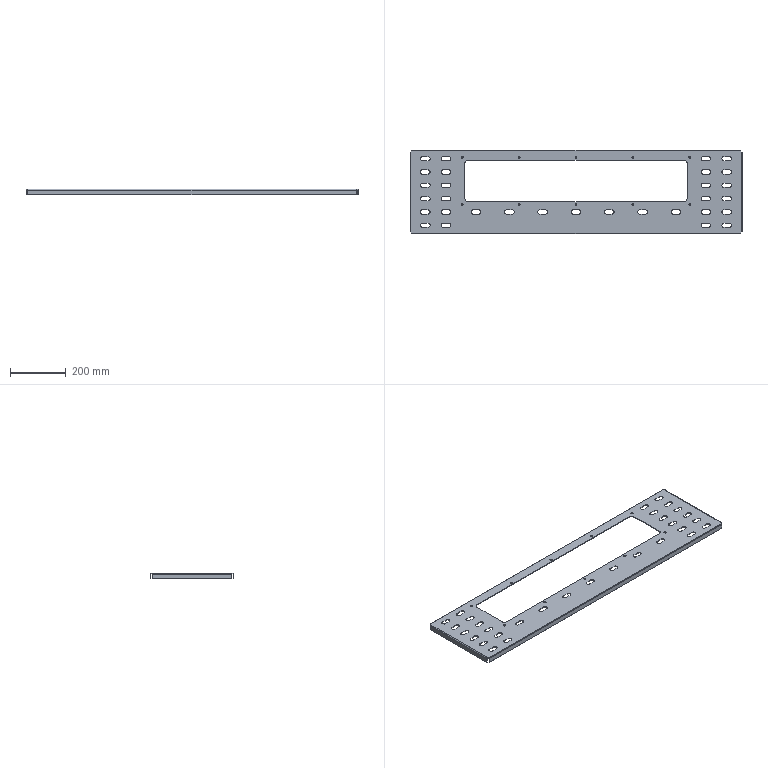Part | SolidWorks | features BaseBody 1 | 1 solid | 333 faces | box 1196 x 302 x 20 mm | volume 691063 mm3 | plane 188 | cylinder 145 | commonest cylinder face diameters 15 x93 6 x24 7 x20 1 x4 20 x4